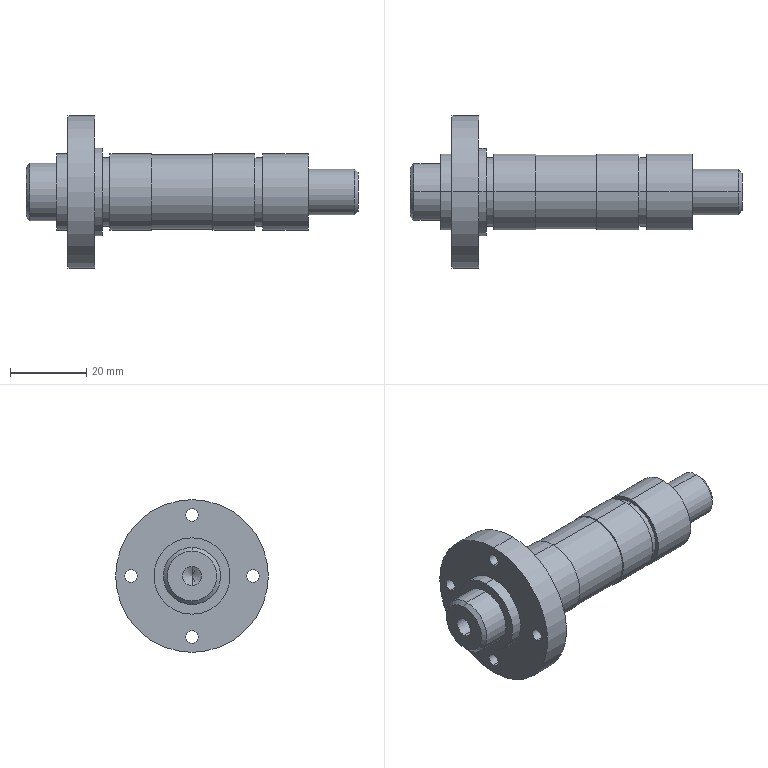Part | SolidWorks | features HoleWzd 2, Chamfer 1, RevCut 1, Revolution 1 | 1 solid | 50 faces | box 87 x 40 x 40 mm | volume 29288 mm3 | cylinder 32 | plane 12 | cone 6 | commonest cylinder face diameters 3.3 x8 20 x8 18 x4 5 x2 12 x2 15 x2
STEP:
#1=CARTESIAN_POINT('',(0.,0.,6.5));
#2=VERTEX_POINT('',#1);
#3=CARTESIAN_POINT('',(0.,0.,-6.5));
#4=VERTEX_POINT('',#3);
#5=CARTESIAN_POINT('',(0.,0.,0.));
#6=DIRECTION('',(-1.,0.,0.));
#7=DIRECTION('',(0.,0.,-1.));
#8=AXIS2_PLACEMENT_3D('',#5,#6,#7);
#9=CIRCLE('',#8,6.5);
#10=EDGE_CURVE('',#2,#4,#9,.T.);
#11=ORIENTED_EDGE('',*,*,#10,.F.);
#12=CARTESIAN_POINT('',(1.,0.,7.5));
#13=VERTEX_POINT('',#12);
#14=CARTESIAN_POINT('',(0.,0.,6.5));
#15=DIRECTION('',(0.7071,0.,0.7071));
#16=VECTOR('',#15,1000.);
#17=LINE('',#14,#16);
#18=EDGE_CURVE('',#2,#13,#17,.T.);
#19=ORIENTED_EDGE('',*,*,#18,.T.);
#20=CARTESIAN_POINT('',(1.,0.,-7.5));
#21=VERTEX_POINT('',#20);
#22=CARTESIAN_POINT('',(1.,0.,0.));
#23=DIRECTION('',(1.,0.,0.));
#24=DIRECTION('',(0.,0.,-1.));
#25=AXIS2_PLACEMENT_3D('',#22,#23,#24);
#26=CIRCLE('',#25,7.5);
#27=EDGE_CURVE('',#21,#13,#26,.T.);
#28=ORIENTED_EDGE('',*,*,#27,.F.);
#29=CARTESIAN_POINT('',(0.,0.,-6.5));
#30=DIRECTION('',(0.7071,0.,-0.7071));
#31=VECTOR('',#30,1000.);
#32=LINE('',#29,#31);
#33=EDGE_CURVE('',#4,#21,#32,.T.);
#34=ORIENTED_EDGE('',*,*,#33,.F.);
#35=EDGE_LOOP('',(#11,#19,#28,#34));
#36=FACE_OUTER_BOUND('',#35,.T.);
#37=CARTESIAN_POINT('',(0.,0.,0.));
#38=DIRECTION('',(1.,0.,0.));
#39=DIRECTION('',(0.,0.,-1.));
#40=AXIS2_PLACEMENT_3D('',#37,#38,#39);
#41=CONICAL_SURFACE('',#40,6.5,0.7854);
#42=ADVANCED_FACE('',(#36),#41,.T.);
#43=CARTESIAN_POINT('',(87.,0.,-5.));
#44=VERTEX_POINT('',#43);
#45=CARTESIAN_POINT('',(87.,0.,5.));
#46=VERTEX_POINT('',#45);
#47=CARTESIAN_POINT('',(87.,0.,0.));
#48=DIRECTION('',(1.,0.,0.));
#49=DIRECTION('',(0.,0.,1.));
#50=AXIS2_PLACEMENT_3D('',#47,#48,#49);
#51=CIRCLE('',#50,5.);
#52=EDGE_CURVE('',#44,#46,#51,.T.);
#53=ORIENTED_EDGE('',*,*,#52,.F.);
#54=CARTESIAN_POINT('',(86.,0.,-6.));
#55=VERTEX_POINT('',#54);
#56=CARTESIAN_POINT('',(86.,0.,-6.));
#57=DIRECTION('',(-0.7071,0.,-0.7071));
#58=VECTOR('',#57,1000.);
#59=LINE('',#56,#58);
#60=EDGE_CURVE('',#44,#55,#59,.T.);
#61=ORIENTED_EDGE('',*,*,#60,.T.);
#62=CARTESIAN_POINT('',(86.,0.,6.));
#63=VERTEX_POINT('',#62);
#64=CARTESIAN_POINT('',(86.,0.,0.));
#65=DIRECTION('',(-1.,0.,0.));
#66=DIRECTION('',(0.,0.,1.));
#67=AXIS2_PLACEMENT_3D('',#64,#65,#66);
#68=CIRCLE('',#67,6.);
#69=EDGE_CURVE('',#63,#55,#68,.T.);
#70=ORIENTED_EDGE('',*,*,#69,.F.);
#71=CARTESIAN_POINT('',(86.,0.,6.));
#72=DIRECTION('',(-0.7071,0.,0.7071));
#73=VECTOR('',#72,1000.);
#74=LINE('',#71,#73);
#75=EDGE_CURVE('',#46,#63,#74,.T.);
#76=ORIENTED_EDGE('',*,*,#75,.F.);
#77=EDGE_LOOP('',(#53,#61,#70,#76));
#78=FACE_OUTER_BOUND('',#77,.T.);
#79=CARTESIAN_POINT('',(86.,0.,0.));
#80=DIRECTION('',(-1.,0.,0.));
#81=DIRECTION('',(0.,0.,1.));
#82=AXIS2_PLACEMENT_3D('',#79,#80,#81);
#83=CONICAL_SURFACE('',#82,6.,0.7854);
#84=ADVANCED_FACE('',(#78),#83,.T.);
#85=CARTESIAN_POINT('',(20.,0.,11.5));
#86=VERTEX_POINT('',#85);
#87=CARTESIAN_POINT('',(20.,0.,-11.5));
#88=VERTEX_POINT('',#87);
#89=CARTESIAN_POINT('',(20.,0.,0.));
#90=DIRECTION('',(-1.,0.,0.));
#91=DIRECTION('',(0.,0.,1.));
#92=AXIS2_PLACEMENT_3D('',#89,#90,#91);
#93=CIRCLE('',#92,11.5);
#94=EDGE_CURVE('',#86,#88,#93,.T.);
#95=ORIENTED_EDGE('',*,*,#94,.T.);
#96=CARTESIAN_POINT('',(18.,0.,-11.5));
#97=VERTEX_POINT('',#96);
#98=CARTESIAN_POINT('',(0.,0.,-11.5));
#99=DIRECTION('',(-1.,0.,0.));
#100=VECTOR('',#99,1000.);
#101=LINE('',#98,#100);
#102=EDGE_CURVE('',#88,#97,#101,.T.);
#103=ORIENTED_EDGE('',*,*,#102,.T.);
#104=CARTESIAN_POINT('',(18.,0.,11.5));
#105=VERTEX_POINT('',#104);
#106=CARTESIAN_POINT('',(18.,0.,0.));
#107=DIRECTION('',(-1.,0.,0.));
#108=DIRECTION('',(0.,0.,1.));
#109=AXIS2_PLACEMENT_3D('',#106,#107,#108);
#110=CIRCLE('',#109,11.5);
#111=EDGE_CURVE('',#105,#97,#110,.T.);
#112=ORIENTED_EDGE('',*,*,#111,.F.);
#113=CARTESIAN_POINT('',(0.,0.,11.5));
#114=DIRECTION('',(-1.,0.,0.));
#115=VECTOR('',#114,1000.);
#116=LINE('',#113,#115);
#117=EDGE_CURVE('',#86,#105,#116,.T.);
#118=ORIENTED_EDGE('',*,*,#117,.F.);
#119=EDGE_LOOP('',(#95,#103,#112,#118));
#120=FACE_OUTER_BOUND('',#119,.T.);
#121=CARTESIAN_POINT('',(0.,0.,0.));
#122=DIRECTION('',(-1.,0.,0.));
#123=DIRECTION('',(0.,0.,1.));
#124=AXIS2_PLACEMENT_3D('',#121,#122,#123);
#125=CYLINDRICAL_SURFACE('',#124,11.5);
#126=ADVANCED_FACE('',(#120),#125,.T.);
#127=CARTESIAN_POINT('',(18.,16.,-1.65));
#128=VERTEX_POINT('',#127);
#129=CARTESIAN_POINT('',(18.,16.,1.65));
#130=VERTEX_POINT('',#129);
#131=CARTESIAN_POINT('',(18.,16.,0.));
#132=DIRECTION('',(-1.,0.,0.));
#133=DIRECTION('',(0.,0.,1.));
#134=AXIS2_PLACEMENT_3D('',#131,#132,#133);
#135=CIRCLE('',#134,1.65);
#136=EDGE_CURVE('',#128,#130,#135,.T.);
#137=ORIENTED_EDGE('',*,*,#136,.F.);
#138=CARTESIAN_POINT('',(11.,16.,-1.65));
#139=VERTEX_POINT('',#138);
#140=CARTESIAN_POINT('',(11.,16.,-1.65));
#141=DIRECTION('',(-1.,0.,0.));
#142=VECTOR('',#141,1000.);
#143=LINE('',#140,#142);
#144=EDGE_CURVE('',#128,#139,#143,.T.);
#145=ORIENTED_EDGE('',*,*,#144,.T.);
#146=CARTESIAN_POINT('',(11.,16.,1.65));
#147=VERTEX_POINT('',#146);
#148=CARTESIAN_POINT('',(11.,16.,0.));
#149=DIRECTION('',(-1.,0.,0.));
#150=DIRECTION('',(0.,0.,1.));
#151=AXIS2_PLACEMENT_3D('',#148,#149,#150);
#152=CIRCLE('',#151,1.65);
#153=EDGE_CURVE('',#139,#147,#152,.T.);
#154=ORIENTED_EDGE('',*,*,#153,.T.);
#155=CARTESIAN_POINT('',(11.,16.,1.65));
#156=DIRECTION('',(-1.,0.,0.));
#157=VECTOR('',#156,1000.);
#158=LINE('',#155,#157);
#159=EDGE_CURVE('',#130,#147,#158,.T.);
#160=ORIENTED_EDGE('',*,*,#159,.F.);
#161=EDGE_LOOP('',(#137,#145,#154,#160));
#162=FACE_OUTER_BOUND('',#161,.T.);
#163=CARTESIAN_POINT('',(11.,16.,0.));
#164=DIRECTION('',(-1.,0.,0.));
#165=DIRECTION('',(0.,0.,1.));
#166=AXIS2_PLACEMENT_3D('',#163,#164,#165);
#167=CYLINDRICAL_SURFACE('',#166,1.65);
#168=ADVANCED_FACE('',(#162),#167,.F.);
#169=CARTESIAN_POINT('',(18.,0.,-17.65));
#170=VERTEX_POINT('',#169);
#171=CARTESIAN_POINT('',(18.,0.,-14.35));
#172=VERTEX_POINT('',#171);
#173=CARTESIAN_POINT('',(18.,0.,-16.));
#174=DIRECTION('',(-1.,0.,0.));
#175=DIRECTION('',(0.,0.,1.));
#176=AXIS2_PLACEMENT_3D('',#173,#174,#175);
#177=CIRCLE('',#176,1.65);
#178=EDGE_CURVE('',#170,#172,#177,.T.);
#179=ORIENTED_EDGE('',*,*,#178,.F.);
#180=CARTESIAN_POINT('',(11.,0.,-17.65));
#181=VERTEX_POINT('',#180);
#182=CARTESIAN_POINT('',(11.,0.,-17.65));
#183=DIRECTION('',(-1.,0.,0.));
#184=VECTOR('',#183,1000.);
#185=LINE('',#182,#184);
#186=EDGE_CURVE('',#170,#181,#185,.T.);
#187=ORIENTED_EDGE('',*,*,#186,.T.);
#188=CARTESIAN_POINT('',(11.,0.,-14.35));
#189=VERTEX_POINT('',#188);
#190=CARTESIAN_POINT('',(11.,0.,-16.));
#191=DIRECTION('',(-1.,0.,0.));
#192=DIRECTION('',(0.,0.,1.));
#193=AXIS2_PLACEMENT_3D('',#190,#191,#192);
#194=CIRCLE('',#193,1.65);
#195=EDGE_CURVE('',#181,#189,#194,.T.);
#196=ORIENTED_EDGE('',*,*,#195,.T.);
#197=CARTESIAN_POINT('',(11.,0.,-14.35));
#198=DIRECTION('',(-1.,0.,0.));
#199=VECTOR('',#198,1000.);
#200=LINE('',#197,#199);
#201=EDGE_CURVE('',#172,#189,#200,.T.);
#202=ORIENTED_EDGE('',*,*,#201,.F.);
#203=EDGE_LOOP('',(#179,#187,#196,#202));
#204=FACE_OUTER_BOUND('',#203,.T.);
#205=CARTESIAN_POINT('',(11.,0.,-16.));
#206=DIRECTION('',(-1.,0.,0.));
#207=DIRECTION('',(0.,0.,1.));
#208=AXIS2_PLACEMENT_3D('',#205,#206,#207);
#209=CYLINDRICAL_SURFACE('',#208,1.65);
#210=ADVANCED_FACE('',(#204),#209,.F.);
#211=CARTESIAN_POINT('',(18.,-16.,-1.65));
#212=VERTEX_POINT('',#211);
#213=CARTESIAN_POINT('',(18.,-16.,1.65));
#214=VERTEX_POINT('',#213);
#215=CARTESIAN_POINT('',(18.,-16.,0.));
#216=DIRECTION('',(-1.,0.,0.));
#217=DIRECTION('',(0.,0.,1.));
#218=AXIS2_PLACEMENT_3D('',#215,#216,#217);
#219=CIRCLE('',#218,1.65);
#220=EDGE_CURVE('',#212,#214,#219,.T.);
#221=ORIENTED_EDGE('',*,*,#220,.F.);
#222=CARTESIAN_POINT('',(11.,-16.,-1.65));
#223=VERTEX_POINT('',#222);
#224=CARTESIAN_POINT('',(11.,-16.,-1.65));
#225=DIRECTION('',(-1.,0.,0.));
#226=VECTOR('',#225,1000.);
#227=LINE('',#224,#226);
#228=EDGE_CURVE('',#212,#223,#227,.T.);
#229=ORIENTED_EDGE('',*,*,#228,.T.);
#230=CARTESIAN_POINT('',(11.,-16.,1.65));
#231=VERTEX_POINT('',#230);
#232=CARTESIAN_POINT('',(11.,-16.,0.));
#233=DIRECTION('',(-1.,0.,0.));
#234=DIRECTION('',(0.,0.,1.));
#235=AXIS2_PLACEMENT_3D('',#232,#233,#234);
#236=CIRCLE('',#235,1.65);
#237=EDGE_CURVE('',#223,#231,#236,.T.);
#238=ORIENTED_EDGE('',*,*,#237,.T.);
#239=CARTESIAN_POINT('',(11.,-16.,1.65));
#240=DIRECTION('',(-1.,0.,0.));
#241=VECTOR('',#240,1000.);
#242=LINE('',#239,#241);
#243=EDGE_CURVE('',#214,#231,#242,.T.);
#244=ORIENTED_EDGE('',*,*,#243,.F.);
#245=EDGE_LOOP('',(#221,#229,#238,#244));
#246=FACE_OUTER_BOUND('',#245,.T.);
#247=CARTESIAN_POINT('',(11.,-16.,0.));
#248=DIRECTION('',(-1.,0.,0.));
#249=DIRECTION('',(0.,0.,1.));
#250=AXIS2_PLACEMENT_3D('',#247,#248,#249);
#251=CYLINDRICAL_SURFACE('',#250,1.65);
#252=ADVANCED_FACE('',(#246),#251,.F.);
#253=CARTESIAN_POINT('',(18.,0.,14.35));
#254=VERTEX_POINT('',#253);
#255=CARTESIAN_POINT('',(18.,0.,17.65));
#256=VERTEX_POINT('',#255);
#257=CARTESIAN_POINT('',(18.,0.,16.));
#258=DIRECTION('',(-1.,0.,0.));
#259=DIRECTION('',(0.,0.,1.));
#260=AXIS2_PLACEMENT_3D('',#257,#258,#259);
#261=CIRCLE('',#260,1.65);
#262=EDGE_CURVE('',#254,#256,#261,.T.);
#263=ORIENTED_EDGE('',*,*,#262,.F.);
#264=CARTESIAN_POINT('',(11.,0.,14.35));
#265=VERTEX_POINT('',#264);
#266=CARTESIAN_POINT('',(11.,0.,14.35));
#267=DIRECTION('',(-1.,0.,0.));
#268=VECTOR('',#267,1000.);
#269=LINE('',#266,#268);
#270=EDGE_CURVE('',#254,#265,#269,.T.);
#271=ORIENTED_EDGE('',*,*,#270,.T.);
#272=CARTESIAN_POINT('',(11.,0.,17.65));
#273=VERTEX_POINT('',#272);
#274=CARTESIAN_POINT('',(11.,0.,16.));
#275=DIRECTION('',(-1.,0.,0.));
#276=DIRECTION('',(0.,0.,1.));
#277=AXIS2_PLACEMENT_3D('',#274,#275,#276);
#278=CIRCLE('',#277,1.65);
#279=EDGE_CURVE('',#265,#273,#278,.T.);
#280=ORIENTED_EDGE('',*,*,#279,.T.);
#281=CARTESIAN_POINT('',(11.,0.,17.65));
#282=DIRECTION('',(-1.,0.,0.));
#283=VECTOR('',#282,1000.);
#284=LINE('',#281,#283);
#285=EDGE_CURVE('',#256,#273,#284,.T.);
#286=ORIENTED_EDGE('',*,*,#285,.F.);
#287=EDGE_LOOP('',(#263,#271,#280,#286));
#288=FACE_OUTER_BOUND('',#287,.T.);
#289=CARTESIAN_POINT('',(11.,0.,16.));
#290=DIRECTION('',(-1.,0.,0.));
#291=DIRECTION('',(0.,0.,1.));
#292=AXIS2_PLACEMENT_3D('',#289,#290,#291);
#293=CYLINDRICAL_SURFACE('',#292,1.65);
#294=ADVANCED_FACE('',(#288),#293,.F.);
#295=CARTESIAN_POINT('',(18.,0.,20.));
#296=VERTEX_POINT('',#295);
#297=CARTESIAN_POINT('',(18.,0.,-20.));
#298=VERTEX_POINT('',#297);
#299=CARTESIAN_POINT('',(18.,0.,0.));
#300=DIRECTION('',(-1.,0.,0.));
#301=DIRECTION('',(0.,0.,1.));
#302=AXIS2_PLACEMENT_3D('',#299,#300,#301);
#303=CIRCLE('',#302,20.);
#304=EDGE_CURVE('',#296,#298,#303,.T.);
#305=ORIENTED_EDGE('',*,*,#304,.T.);
#306=CARTESIAN_POINT('',(11.,0.,-20.));
#307=VERTEX_POINT('',#306);
#308=CARTESIAN_POINT('',(0.,0.,-20.));
#309=DIRECTION('',(-1.,0.,0.));
#310=VECTOR('',#309,1000.);
#311=LINE('',#308,#310);
#312=EDGE_CURVE('',#298,#307,#311,.T.);
#313=ORIENTED_EDGE('',*,*,#312,.T.);
#314=CARTESIAN_POINT('',(11.,0.,20.));
#315=VERTEX_POINT('',#314);
#316=CARTESIAN_POINT('',(11.,0.,0.));
#317=DIRECTION('',(-1.,0.,0.));
#318=DIRECTION('',(0.,0.,1.));
#319=AXIS2_PLACEMENT_3D('',#316,#317,#318);
#320=CIRCLE('',#319,20.);
#321=EDGE_CURVE('',#315,#307,#320,.T.);
#322=ORIENTED_EDGE('',*,*,#321,.F.);
#323=CARTESIAN_POINT('',(0.,0.,20.));
#324=DIRECTION('',(-1.,0.,0.));
#325=VECTOR('',#324,1000.);
#326=LINE('',#323,#325);
#327=EDGE_CURVE('',#296,#315,#326,.T.);
#328=ORIENTED_EDGE('',*,*,#327,.F.);
#329=EDGE_LOOP('',(#305,#313,#322,#328));
#330=FACE_OUTER_BOUND('',#329,.T.);
#331=CARTESIAN_POINT('',(0.,0.,0.));
#332=DIRECTION('',(-1.,0.,0.));
#333=DIRECTION('',(0.,0.,1.));
#334=AXIS2_PLACEMENT_3D('',#331,#332,#333);
#335=CYLINDRICAL_SURFACE('',#334,20.);
#336=ADVANCED_FACE('',(#330),#335,.T.);
#337=CARTESIAN_POINT('',(11.,0.,10.));
#338=VERTEX_POINT('',#337);
#339=CARTESIAN_POINT('',(11.,0.,-10.));
#340=VERTEX_POINT('',#339);
#341=CARTESIAN_POINT('',(11.,0.,0.));
#342=DIRECTION('',(-1.,0.,0.));
#343=DIRECTION('',(0.,0.,1.));
#344=AXIS2_PLACEMENT_3D('',#341,#342,#343);
#345=CIRCLE('',#344,10.);
#346=EDGE_CURVE('',#338,#340,#345,.T.);
#347=ORIENTED_EDGE('',*,*,#346,.T.);
#348=CARTESIAN_POINT('',(8.,0.,-10.));
#349=VERTEX_POINT('',#348);
#350=CARTESIAN_POINT('',(0.,0.,-10.));
#351=DIRECTION('',(-1.,0.,0.));
#352=VECTOR('',#351,1000.);
#353=LINE('',#350,#352);
#354=EDGE_CURVE('',#340,#349,#353,.T.);
#355=ORIENTED_EDGE('',*,*,#354,.T.);
#356=CARTESIAN_POINT('',(8.,0.,10.));
#357=VERTEX_POINT('',#356);
#358=CARTESIAN_POINT('',(8.,0.,0.));
#359=DIRECTION('',(-1.,0.,0.));
#360=DIRECTION('',(0.,0.,1.));
#361=AXIS2_PLACEMENT_3D('',#358,#359,#360);
#362=CIRCLE('',#361,10.);
#363=EDGE_CURVE('',#357,#349,#362,.T.);
#364=ORIENTED_EDGE('',*,*,#363,.F.);
#365=CARTESIAN_POINT('',(0.,0.,10.));
#366=DIRECTION('',(-1.,0.,0.));
#367=VECTOR('',#366,1000.);
#368=LINE('',#365,#367);
#369=EDGE_CURVE('',#338,#357,#368,.T.);
#370=ORIENTED_EDGE('',*,*,#369,.F.);
#371=EDGE_LOOP('',(#347,#355,#364,#370));
#372=FACE_OUTER_BOUND('',#371,.T.);
#373=CARTESIAN_POINT('',(0.,0.,0.));
#374=DIRECTION('',(-1.,0.,0.));
#375=DIRECTION('',(0.,0.,1.));
#376=AXIS2_PLACEMENT_3D('',#373,#374,#375);
#377=CYLINDRICAL_SURFACE('',#376,10.);
#378=ADVANCED_FACE('',(#372),#377,.T.);
#379=CARTESIAN_POINT('',(8.,0.,7.5));
#380=VERTEX_POINT('',#379);
#381=CARTESIAN_POINT('',(8.,0.,-7.5));
#382=VERTEX_POINT('',#381);
#383=CARTESIAN_POINT('',(8.,0.,0.));
#384=DIRECTION('',(-1.,0.,0.));
#385=DIRECTION('',(0.,0.,1.));
#386=AXIS2_PLACEMENT_3D('',#383,#384,#385);
#387=CIRCLE('',#386,7.5);
#388=EDGE_CURVE('',#380,#382,#387,.T.);
#389=ORIENTED_EDGE('',*,*,#388,.T.);
#390=CARTESIAN_POINT('',(0.,0.,-7.5));
#391=DIRECTION('',(-1.,0.,0.));
#392=VECTOR('',#391,1000.);
#393=LINE('',#390,#392);
#394=EDGE_CURVE('',#382,#21,#393,.T.);
#395=ORIENTED_EDGE('',*,*,#394,.T.);
#396=ORIENTED_EDGE('',*,*,#27,.T.);
#397=CARTESIAN_POINT('',(0.,0.,7.5));
#398=DIRECTION('',(-1.,0.,0.));
#399=VECTOR('',#398,1000.);
#400=LINE('',#397,#399);
#401=EDGE_CURVE('',#380,#13,#400,.T.);
#402=ORIENTED_EDGE('',*,*,#401,.F.);
#403=EDGE_LOOP('',(#389,#395,#396,#402));
#404=FACE_OUTER_BOUND('',#403,.T.);
#405=CARTESIAN_POINT('',(0.,0.,0.));
#406=DIRECTION('',(-1.,0.,0.));
#407=DIRECTION('',(0.,0.,1.));
#408=AXIS2_PLACEMENT_3D('',#405,#406,#407);
#409=CYLINDRICAL_SURFACE('',#408,7.5);
#410=ADVANCED_FACE('',(#404),#409,.T.);
#411=CARTESIAN_POINT('',(18.,0.,-2.5));
#412=VERTEX_POINT('',#411);
#413=CARTESIAN_POINT('',(18.,0.,2.5));
#414=VERTEX_POINT('',#413);
#415=CARTESIAN_POINT('',(18.,0.,0.));
#416=DIRECTION('',(-1.,0.,0.));
#417=DIRECTION('',(0.,0.,1.));
#418=AXIS2_PLACEMENT_3D('',#415,#416,#417);
#419=CIRCLE('',#418,2.5);
#420=EDGE_CURVE('',#412,#414,#419,.T.);
#421=ORIENTED_EDGE('',*,*,#420,.F.);
#422=CARTESIAN_POINT('',(0.,0.,-2.5));
#423=VERTEX_POINT('',#422);
#424=CARTESIAN_POINT('',(0.,0.,-2.5));
#425=DIRECTION('',(-1.,0.,0.));
#426=VECTOR('',#425,1000.);
#427=LINE('',#424,#426);
#428=EDGE_CURVE('',#412,#423,#427,.T.);
#429=ORIENTED_EDGE('',*,*,#428,.T.);
#430=CARTESIAN_POINT('',(0.,0.,2.5));
#431=VERTEX_POINT('',#430);
#432=CARTESIAN_POINT('',(0.,0.,0.));
#433=DIRECTION('',(-1.,0.,0.));
#434=DIRECTION('',(0.,0.,1.));
#435=AXIS2_PLACEMENT_3D('',#432,#433,#434);
#436=CIRCLE('',#435,2.5);
#437=EDGE_CURVE('',#423,#431,#436,.T.);
#438=ORIENTED_EDGE('',*,*,#437,.T.);
#439=CARTESIAN_POINT('',(0.,0.,2.5));
#440=DIRECTION('',(-1.,0.,0.));
#441=VECTOR('',#440,1000.);
#442=LINE('',#439,#441);
#443=EDGE_CURVE('',#414,#431,#442,.T.);
#444=ORIENTED_EDGE('',*,*,#443,.F.);
#445=EDGE_LOOP('',(#421,#429,#438,#444));
#446=FACE_OUTER_BOUND('',#445,.T.);
#447=CARTESIAN_POINT('',(0.,0.,0.));
#448=DIRECTION('',(-1.,0.,0.));
#449=DIRECTION('',(0.,0.,1.));
#450=AXIS2_PLACEMENT_3D('',#447,#448,#449);
#451=CYLINDRICAL_SURFACE('',#450,2.5);
#452=ADVANCED_FACE('',(#446),#451,.F.);
#453=CARTESIAN_POINT('',(19.502,0.,0.));
#454=VERTEX_POINT('',#453);
#455=CARTESIAN_POINT('',(18.,0.,2.5));
#456=DIRECTION('',(-0.515,0.,0.8572));
#457=VECTOR('',#456,1000.);
#458=LINE('',#455,#457);
#459=EDGE_CURVE('',#454,#414,#458,.T.);
#460=ORIENTED_EDGE('',*,*,#459,.F.);
#461=CARTESIAN_POINT('',(18.,0.,-2.5));
#462=DIRECTION('',(-0.515,0.,-0.8572));
#463=VECTOR('',#462,1000.);
#464=LINE('',#461,#463);
#465=EDGE_CURVE('',#454,#412,#464,.T.);
#466=ORIENTED_EDGE('',*,*,#465,.T.);
#467=ORIENTED_EDGE('',*,*,#420,.T.);
#468=EDGE_LOOP('',(#460,#466,#467));
#469=FACE_OUTER_BOUND('',#468,.T.);
#470=CARTESIAN_POINT('',(18.,0.,0.));
#471=DIRECTION('',(-1.,0.,0.));
#472=DIRECTION('',(0.,0.,1.));
#473=AXIS2_PLACEMENT_3D('',#470,#471,#472);
#474=CONICAL_SURFACE('',#473,2.5,1.03);
#475=ADVANCED_FACE('',(#469),#474,.F.);
#476=CARTESIAN_POINT('',(22.,0.,9.));
#477=VERTEX_POINT('',#476);
#478=CARTESIAN_POINT('',(22.,0.,-9.));
#479=VERTEX_POINT('',#478);
#480=CARTESIAN_POINT('',(22.,0.,0.));
#481=DIRECTION('',(-1.,0.,0.));
#482=DIRECTION('',(0.,0.,1.));
#483=AXIS2_PLACEMENT_3D('',#480,#481,#482);
#484=CIRCLE('',#483,9.);
#485=EDGE_CURVE('',#477,#479,#484,.T.);
#486=ORIENTED_EDGE('',*,*,#485,.T.);
#487=CARTESIAN_POINT('',(20.,0.,-9.));
#488=VERTEX_POINT('',#487);
#489=CARTESIAN_POINT('',(0.,0.,-9.));
#490=DIRECTION('',(-1.,0.,0.));
#491=VECTOR('',#490,1000.);
#492=LINE('',#489,#491);
#493=EDGE_CURVE('',#479,#488,#492,.T.);
#494=ORIENTED_EDGE('',*,*,#493,.T.);
#495=CARTESIAN_POINT('',(20.,0.,9.));
#496=VERTEX_POINT('',#495);
#497=CARTESIAN_POINT('',(20.,0.,0.));
#498=DIRECTION('',(-1.,0.,0.));
#499=DIRECTION('',(0.,0.,1.));
#500=AXIS2_PLACEMENT_3D('',#497,#498,#499);
#501=CIRCLE('',#500,9.);
#502=EDGE_CURVE('',#496,#488,#501,.T.);
#503=ORIENTED_EDGE('',*,*,#502,.F.);
#504=CARTESIAN_POINT('',(0.,0.,9.));
#505=DIRECTION('',(-1.,0.,0.));
#506=VECTOR('',#505,1000.);
#507=LINE('',#504,#506);
#508=EDGE_CURVE('',#477,#496,#507,.T.);
#509=ORIENTED_EDGE('',*,*,#508,.F.);
#510=EDGE_LOOP('',(#486,#494,#503,#509));
#511=FACE_OUTER_BOUND('',#510,.T.);
#512=CARTESIAN_POINT('',(0.,0.,0.));
#513=DIRECTION('',(-1.,0.,0.));
#514=DIRECTION('',(0.,0.,1.));
#515=AXIS2_PLACEMENT_3D('',#512,#513,#514);
#516=CYLINDRICAL_SURFACE('',#515,9.);
#517=ADVANCED_FACE('',(#511),#516,.T.);
#518=ORIENTED_EDGE('',*,*,#69,.T.);
#519=CARTESIAN_POINT('',(74.,0.,-6.));
#520=VERTEX_POINT('',#519);
#521=CARTESIAN_POINT('',(0.,0.,-6.));
#522=DIRECTION('',(-1.,0.,0.));
#523=VECTOR('',#522,1000.);
#524=LINE('',#521,#523);
#525=EDGE_CURVE('',#55,#520,#524,.T.);
#526=ORIENTED_EDGE('',*,*,#525,.T.);
#527=CARTESIAN_POINT('',(74.,0.,6.));
#528=VERTEX_POINT('',#527);
#529=CARTESIAN_POINT('',(74.,0.,0.));
#530=DIRECTION('',(-1.,0.,0.));
#531=DIRECTION('',(0.,0.,1.));
#532=AXIS2_PLACEMENT_3D('',#529,#530,#531);
#533=CIRCLE('',#532,6.);
#534=EDGE_CURVE('',#528,#520,#533,.T.);
#535=ORIENTED_EDGE('',*,*,#534,.F.);
#536=CARTESIAN_POINT('',(0.,0.,6.));
#537=DIRECTION('',(-1.,0.,0.));
#538=VECTOR('',#537,1000.);
#539=LINE('',#536,#538);
#540=EDGE_CURVE('',#63,#528,#539,.T.);
#541=ORIENTED_EDGE('',*,*,#540,.F.);
#542=EDGE_LOOP('',(#518,#526,#535,#541));
#543=FACE_OUTER_BOUND('',#542,.T.);
#544=CARTESIAN_POINT('',(0.,0.,0.));
#545=DIRECTION('',(-1.,0.,0.));
#546=DIRECTION('',(0.,0.,1.));
#547=AXIS2_PLACEMENT_3D('',#544,#545,#546);
#548=CYLINDRICAL_SURFACE('',#547,6.);
#549=ADVANCED_FACE('',(#543),#548,.T.);
#550=CARTESIAN_POINT('',(74.,0.,10.));
#551=VERTEX_POINT('',#550);
#552=CARTESIAN_POINT('',(74.,0.,-10.));
#553=VERTEX_POINT('',#552);
#554=CARTESIAN_POINT('',(74.,0.,0.));
#555=DIRECTION('',(-1.,0.,0.));
#556=DIRECTION('',(0.,0.,1.));
#557=AXIS2_PLACEMENT_3D('',#554,#555,#556);
#558=CIRCLE('',#557,10.);
#559=EDGE_CURVE('',#551,#553,#558,.T.);
#560=ORIENTED_EDGE('',*,*,#559,.T.);
#561=CARTESIAN_POINT('',(62.,0.,-10.));
#562=VERTEX_POINT('',#561);
#563=CARTESIAN_POINT('',(0.,0.,-10.));
#564=DIRECTION('',(-1.,0.,0.));
#565=VECTOR('',#564,1000.);
#566=LINE('',#563,#565);
#567=EDGE_CURVE('',#553,#562,#566,.T.);
#568=ORIENTED_EDGE('',*,*,#567,.T.);
#569=CARTESIAN_POINT('',(62.,0.,10.));
#570=VERTEX_POINT('',#569);
#571=CARTESIAN_POINT('',(62.,0.,0.));
#572=DIRECTION('',(-1.,0.,0.));
#573=DIRECTION('',(0.,0.,1.));
#574=AXIS2_PLACEMENT_3D('',#571,#572,#573);
#575=CIRCLE('',#574,10.);
#576=EDGE_CURVE('',#570,#562,#575,.T.);
#577=ORIENTED_EDGE('',*,*,#576,.F.);
#578=CARTESIAN_POINT('',(0.,0.,10.));
#579=DIRECTION('',(-1.,0.,0.));
#580=VECTOR('',#579,1000.);
#581=LINE('',#578,#580);
#582=EDGE_CURVE('',#551,#570,#581,.T.);
#583=ORIENTED_EDGE('',*,*,#582,.F.);
#584=EDGE_LOOP('',(#560,#568,#577,#583));
#585=FACE_OUTER_BOUND('',#584,.T.);
#586=CARTESIAN_POINT('',(0.,0.,0.));
#587=DIRECTION('',(-1.,0.,0.));
#588=DIRECTION('',(0.,0.,1.));
#589=AXIS2_PLACEMENT_3D('',#586,#587,#588);
#590=CYLINDRICAL_SURFACE('',#589,10.);
#591=ADVANCED_FACE('',(#585),#590,.T.);
#592=CARTESIAN_POINT('',(62.,0.,9.));
#593=VERTEX_POINT('',#592);
#594=CARTESIAN_POINT('',(62.,0.,-9.));
#595=VERTEX_POINT('',#594);
#596=CARTESIAN_POINT('',(62.,0.,0.));
#597=DIRECTION('',(-1.,0.,0.));
#598=DIRECTION('',(0.,0.,1.));
#599=AXIS2_PLACEMENT_3D('',#596,#597,#598);
#600=CIRCLE('',#599,9.);
#601=EDGE_CURVE('',#593,#595,#600,.T.);
#602=ORIENTED_EDGE('',*,*,#601,.T.);
#603=CARTESIAN_POINT('',(60.,0.,-9.));
#604=VERTEX_POINT('',#603);
#605=CARTESIAN_POINT('',(0.,0.,-9.));
#606=DIRECTION('',(-1.,0.,0.));
#607=VECTOR('',#606,1000.);
#608=LINE('',#605,#607);
#609=EDGE_CURVE('',#595,#604,#608,.T.);
#610=ORIENTED_EDGE('',*,*,#609,.T.);
#611=CARTESIAN_POINT('',(60.,0.,9.));
#612=VERTEX_POINT('',#611);
#613=CARTESIAN_POINT('',(60.,0.,0.));
#614=DIRECTION('',(-1.,0.,0.));
#615=DIRECTION('',(0.,0.,1.));
#616=AXIS2_PLACEMENT_3D('',#613,#614,#615);
#617=CIRCLE('',#616,9.);
#618=EDGE_CURVE('',#612,#604,#617,.T.);
#619=ORIENTED_EDGE('',*,*,#618,.F.);
#620=CARTESIAN_POINT('',(0.,0.,9.));
#621=DIRECTION('',(-1.,0.,0.));
#622=VECTOR('',#621,1000.);
#623=LINE('',#620,#622);
#624=EDGE_CURVE('',#593,#612,#623,.T.);
#625=ORIENTED_EDGE('',*,*,#624,.F.);
#626=EDGE_LOOP('',(#602,#610,#619,#625));
#627=FACE_OUTER_BOUND('',#626,.T.);
#628=CARTESIAN_POINT('',(0.,0.,0.));
#629=DIRECTION('',(-1.,0.,0.));
#630=DIRECTION('',(0.,0.,1.));
#631=AXIS2_PLACEMENT_3D('',#628,#629,#630);
#632=CYLINDRICAL_SURFACE('',#631,9.);
#633=ADVANCED_FACE('',(#627),#632,.T.);
#634=CARTESIAN_POINT('',(60.,0.,10.));
#635=VERTEX_POINT('',#634);
#636=CARTESIAN_POINT('',(60.,0.,-10.));
#637=VERTEX_POINT('',#636);
#638=CARTESIAN_POINT('',(60.,0.,0.));
#639=DIRECTION('',(-1.,0.,0.));
#640=DIRECTION('',(0.,0.,1.));
#641=AXIS2_PLACEMENT_3D('',#638,#639,#640);
#642=CIRCLE('',#641,10.);
#643=EDGE_CURVE('',#635,#637,#642,.T.);
#644=ORIENTED_EDGE('',*,*,#643,.T.);
#645=CARTESIAN_POINT('',(49.,0.,-10.));
#646=VERTEX_POINT('',#645);
#647=CARTESIAN_POINT('',(0.,0.,-10.));
#648=DIRECTION('',(-1.,0.,0.));
#649=VECTOR('',#648,1000.);
#650=LINE('',#647,#649);
#651=EDGE_CURVE('',#637,#646,#650,.T.);
#652=ORIENTED_EDGE('',*,*,#651,.T.);
#653=CARTESIAN_POINT('',(49.,0.,10.));
#654=VERTEX_POINT('',#653);
#655=CARTESIAN_POINT('',(49.,0.,0.));
#656=DIRECTION('',(-1.,0.,0.));
#657=DIRECTION('',(0.,0.,1.));
#658=AXIS2_PLACEMENT_3D('',#655,#656,#657);
#659=CIRCLE('',#658,10.);
#660=EDGE_CURVE('',#654,#646,#659,.T.);
#661=ORIENTED_EDGE('',*,*,#660,.F.);
#662=CARTESIAN_POINT('',(0.,0.,10.));
#663=DIRECTION('',(-1.,0.,0.));
#664=VECTOR('',#663,1000.);
#665=LINE('',#662,#664);
#666=EDGE_CURVE('',#635,#654,#665,.T.);
#667=ORIENTED_EDGE('',*,*,#666,.F.);
#668=EDGE_LOOP('',(#644,#652,#661,#667));
#669=FACE_OUTER_BOUND('',#668,.T.);
#670=CARTESIAN_POINT('',(0.,0.,0.));
#671=DIRECTION('',(-1.,0.,0.));
#672=DIRECTION('',(0.,0.,1.));
#673=AXIS2_PLACEMENT_3D('',#670,#671,#672);
#674=CYLINDRICAL_SURFACE('',#673,10.);
#675=ADVANCED_FACE('',(#669),#674,.T.);
#676=CARTESIAN_POINT('',(49.,0.,9.75));
#677=VERTEX_POINT('',#676);
#678=CARTESIAN_POINT('',(49.,0.,-9.75));
#679=VERTEX_POINT('',#678);
#680=CARTESIAN_POINT('',(49.,0.,0.));
#681=DIRECTION('',(-1.,0.,0.));
#682=DIRECTION('',(0.,0.,1.));
#683=AXIS2_PLACEMENT_3D('',#680,#681,#682);
#684=CIRCLE('',#683,9.75);
#685=EDGE_CURVE('',#677,#679,#684,.T.);
#686=ORIENTED_EDGE('',*,*,#685,.T.);
#687=CARTESIAN_POINT('',(33.,0.,-9.75));
#688=VERTEX_POINT('',#687);
#689=CARTESIAN_POINT('',(0.,0.,-9.75));
#690=DIRECTION('',(-1.,0.,0.));
#691=VECTOR('',#690,1000.);
#692=LINE('',#689,#691);
#693=EDGE_CURVE('',#679,#688,#692,.T.);
#694=ORIENTED_EDGE('',*,*,#693,.T.);
#695=CARTESIAN_POINT('',(33.,0.,9.75));
#696=VERTEX_POINT('',#695);
#697=CARTESIAN_POINT('',(33.,0.,0.));
#698=DIRECTION('',(-1.,0.,0.));
#699=DIRECTION('',(0.,0.,1.));
#700=AXIS2_PLACEMENT_3D('',#697,#698,#699);
#701=CIRCLE('',#700,9.75);
#702=EDGE_CURVE('',#696,#688,#701,.T.);
#703=ORIENTED_EDGE('',*,*,#702,.F.);
#704=CARTESIAN_POINT('',(0.,0.,9.75));
#705=DIRECTION('',(-1.,0.,0.));
#706=VECTOR('',#705,1000.);
#707=LINE('',#704,#706);
#708=EDGE_CURVE('',#677,#696,#707,.T.);
#709=ORIENTED_EDGE('',*,*,#708,.F.);
#710=EDGE_LOOP('',(#686,#694,#703,#709));
#711=FACE_OUTER_BOUND('',#710,.T.);
#712=CARTESIAN_POINT('',(0.,0.,0.));
#713=DIRECTION('',(-1.,0.,0.));
#714=DIRECTION('',(0.,0.,1.));
#715=AXIS2_PLACEMENT_3D('',#712,#713,#714);
#716=CYLINDRICAL_SURFACE('',#715,9.75);
#717=ADVANCED_FACE('',(#711),#716,.T.);
#718=CARTESIAN_POINT('',(33.,0.,10.));
#719=VERTEX_POINT('',#718);
#720=CARTESIAN_POINT('',(33.,0.,-10.));
#721=VERTEX_POINT('',#720);
#722=CARTESIAN_POINT('',(33.,0.,0.));
#723=DIRECTION('',(-1.,0.,0.));
#724=DIRECTION('',(0.,0.,1.));
#725=AXIS2_PLACEMENT_3D('',#722,#723,#724);
#726=CIRCLE('',#725,10.);
#727=EDGE_CURVE('',#719,#721,#726,.T.);
#728=ORIENTED_EDGE('',*,*,#727,.T.);
#729=CARTESIAN_POINT('',(22.,0.,-10.));
#730=VERTEX_POINT('',#729);
#731=CARTESIAN_POINT('',(0.,0.,-10.));
#732=DIRECTION('',(-1.,0.,0.));
#733=VECTOR('',#732,1000.);
#734=LINE('',#731,#733);
#735=EDGE_CURVE('',#721,#730,#734,.T.);
#736=ORIENTED_EDGE('',*,*,#735,.T.);
#737=CARTESIAN_POINT('',(22.,0.,10.));
#738=VERTEX_POINT('',#737);
#739=CARTESIAN_POINT('',(22.,0.,0.));
#740=DIRECTION('',(-1.,0.,0.));
#741=DIRECTION('',(0.,0.,1.));
#742=AXIS2_PLACEMENT_3D('',#739,#740,#741);
#743=CIRCLE('',#742,10.);
#744=EDGE_CURVE('',#738,#730,#743,.T.);
#745=ORIENTED_EDGE('',*,*,#744,.F.);
#746=CARTESIAN_POINT('',(0.,0.,10.));
#747=DIRECTION('',(-1.,0.,0.));
#748=VECTOR('',#747,1000.);
#749=LINE('',#746,#748);
#750=EDGE_CURVE('',#719,#738,#749,.T.);
#751=ORIENTED_EDGE('',*,*,#750,.F.);
#752=EDGE_LOOP('',(#728,#736,#745,#751));
#753=FACE_OUTER_BOUND('',#752,.T.);
#754=CARTESIAN_POINT('',(0.,0.,0.));
#755=DIRECTION('',(-1.,0.,0.));
#756=DIRECTION('',(0.,0.,1.));
#757=AXIS2_PLACEMENT_3D('',#754,#755,#756);
#758=CYLINDRICAL_SURFACE('',#757,10.);
#759=ADVANCED_FACE('',(#753),#758,.T.);
#760=ORIENTED_EDGE('',*,*,#735,.F.);
#761=CARTESIAN_POINT('',(33.,0.,0.));
#762=DIRECTION('',(-1.,0.,0.));
#763=DIRECTION('',(0.,0.,1.));
#764=AXIS2_PLACEMENT_3D('',#761,#762,#763);
#765=CIRCLE('',#764,10.);
#766=EDGE_CURVE('',#721,#719,#765,.T.);
#767=ORIENTED_EDGE('',*,*,#766,.T.);
#768=ORIENTED_EDGE('',*,*,#750,.T.);
#769=CARTESIAN_POINT('',(22.,0.,0.));
#770=DIRECTION('',(-1.,0.,0.));
#771=DIRECTION('',(0.,0.,1.));
#772=AXIS2_PLACEMENT_3D('',#769,#770,#771);
#773=CIRCLE('',#772,10.);
#774=EDGE_CURVE('',#730,#738,#773,.T.);
#775=ORIENTED_EDGE('',*,*,#774,.F.);
#776=EDGE_LOOP('',(#760,#767,#768,#775));
#777=FACE_OUTER_BOUND('',#776,.T.);
#778=CARTESIAN_POINT('',(0.,0.,0.));
#779=DIRECTION('',(-1.,0.,0.));
#780=DIRECTION('',(0.,0.,1.));
#781=AXIS2_PLACEMENT_3D('',#778,#779,#780);
#782=CYLINDRICAL_SURFACE('',#781,10.);
#783=ADVANCED_FACE('',(#777),#782,.T.);
#784=ORIENTED_EDGE('',*,*,#727,.F.);
#785=ORIENTED_EDGE('',*,*,#766,.F.);
#786=EDGE_LOOP('',(#784,#785));
#787=FACE_OUTER_BOUND('',#786,.T.);
#788=ORIENTED_EDGE('',*,*,#702,.T.);
#789=CARTESIAN_POINT('',(33.,0.,0.));
#790=DIRECTION('',(-1.,0.,0.));
#791=DIRECTION('',(0.,0.,1.));
#792=AXIS2_PLACEMENT_3D('',#789,#790,#791);
#793=CIRCLE('',#792,9.75);
#794=EDGE_CURVE('',#688,#696,#793,.T.);
#795=ORIENTED_EDGE('',*,*,#794,.T.);
#796=EDGE_LOOP('',(#788,#795));
#797=FACE_BOUND('',#796,.T.);
#798=CARTESIAN_POINT('',(33.,10.,0.));
#799=DIRECTION('',(-1.,0.,0.));
#800=DIRECTION('',(0.,0.,1.));
#801=AXIS2_PLACEMENT_3D('',#798,#799,#800);
#802=PLANE('',#801);
#803=ADVANCED_FACE('',(#787,#797),#802,.F.);
#804=ORIENTED_EDGE('',*,*,#693,.F.);
#805=CARTESIAN_POINT('',(49.,0.,0.));
#806=DIRECTION('',(-1.,0.,0.));
#807=DIRECTION('',(0.,0.,1.));
#808=AXIS2_PLACEMENT_3D('',#805,#806,#807);
#809=CIRCLE('',#808,9.75);
#810=EDGE_CURVE('',#679,#677,#809,.T.);
#811=ORIENTED_EDGE('',*,*,#810,.T.);
#812=ORIENTED_EDGE('',*,*,#708,.T.);
#813=ORIENTED_EDGE('',*,*,#794,.F.);
#814=EDGE_LOOP('',(#804,#811,#812,#813));
#815=FACE_OUTER_BOUND('',#814,.T.);
#816=CARTESIAN_POINT('',(0.,0.,0.));
#817=DIRECTION('',(-1.,0.,0.));
#818=DIRECTION('',(0.,0.,1.));
#819=AXIS2_PLACEMENT_3D('',#816,#817,#818);
#820=CYLINDRICAL_SURFACE('',#819,9.75);
#821=ADVANCED_FACE('',(#815),#820,.T.);
#822=ORIENTED_EDGE('',*,*,#685,.F.);
#823=ORIENTED_EDGE('',*,*,#810,.F.);
#824=EDGE_LOOP('',(#822,#823));
#825=FACE_BOUND('',#824,.T.);
#826=ORIENTED_EDGE('',*,*,#660,.T.);
#827=CARTESIAN_POINT('',(49.,0.,0.));
#828=DIRECTION('',(-1.,0.,0.));
#829=DIRECTION('',(0.,0.,1.));
#830=AXIS2_PLACEMENT_3D('',#827,#828,#829);
#831=CIRCLE('',#830,10.);
#832=EDGE_CURVE('',#646,#654,#831,.T.);
#833=ORIENTED_EDGE('',*,*,#832,.T.);
#834=EDGE_LOOP('',(#826,#833));
#835=FACE_OUTER_BOUND('',#834,.T.);
#836=CARTESIAN_POINT('',(49.,9.75,0.));
#837=DIRECTION('',(1.,0.,0.));
#838=DIRECTION('',(0.,0.,-1.));
#839=AXIS2_PLACEMENT_3D('',#836,#837,#838);
#840=PLANE('',#839);
#841=ADVANCED_FACE('',(#825,#835),#840,.F.);
#842=ORIENTED_EDGE('',*,*,#651,.F.);
#843=CARTESIAN_POINT('',(60.,0.,0.));
#844=DIRECTION('',(-1.,0.,0.));
#845=DIRECTION('',(0.,0.,1.));
#846=AXIS2_PLACEMENT_3D('',#843,#844,#845);
#847=CIRCLE('',#846,10.);
#848=EDGE_CURVE('',#637,#635,#847,.T.);
#849=ORIENTED_EDGE('',*,*,#848,.T.);
#850=ORIENTED_EDGE('',*,*,#666,.T.);
#851=ORIENTED_EDGE('',*,*,#832,.F.);
#852=EDGE_LOOP('',(#842,#849,#850,#851));
#853=FACE_OUTER_BOUND('',#852,.T.);
#854=CARTESIAN_POINT('',(0.,0.,0.));
#855=DIRECTION('',(-1.,0.,0.));
#856=DIRECTION('',(0.,0.,1.));
#857=AXIS2_PLACEMENT_3D('',#854,#855,#856);
#858=CYLINDRICAL_SURFACE('',#857,10.);
#859=ADVANCED_FACE('',(#853),#858,.T.);
#860=ORIENTED_EDGE('',*,*,#643,.F.);
#861=ORIENTED_EDGE('',*,*,#848,.F.);
#862=EDGE_LOOP('',(#860,#861));
#863=FACE_OUTER_BOUND('',#862,.T.);
#864=ORIENTED_EDGE('',*,*,#618,.T.);
#865=CARTESIAN_POINT('',(60.,0.,0.));
#866=DIRECTION('',(-1.,0.,0.));
#867=DIRECTION('',(0.,0.,1.));
#868=AXIS2_PLACEMENT_3D('',#865,#866,#867);
#869=CIRCLE('',#868,9.);
#870=EDGE_CURVE('',#604,#612,#869,.T.);
#871=ORIENTED_EDGE('',*,*,#870,.T.);
#872=EDGE_LOOP('',(#864,#871));
#873=FACE_BOUND('',#872,.T.);
#874=CARTESIAN_POINT('',(60.,10.,0.));
#875=DIRECTION('',(-1.,0.,0.));
#876=DIRECTION('',(0.,0.,1.));
#877=AXIS2_PLACEMENT_3D('',#874,#875,#876);
#878=PLANE('',#877);
#879=ADVANCED_FACE('',(#863,#873),#878,.F.);
#880=ORIENTED_EDGE('',*,*,#609,.F.);
#881=CARTESIAN_POINT('',(62.,0.,0.));
#882=DIRECTION('',(-1.,0.,0.));
#883=DIRECTION('',(0.,0.,1.));
#884=AXIS2_PLACEMENT_3D('',#881,#882,#883);
#885=CIRCLE('',#884,9.);
#886=EDGE_CURVE('',#595,#593,#885,.T.);
#887=ORIENTED_EDGE('',*,*,#886,.T.);
#888=ORIENTED_EDGE('',*,*,#624,.T.);
#889=ORIENTED_EDGE('',*,*,#870,.F.);
#890=EDGE_LOOP('',(#880,#887,#888,#889));
#891=FACE_OUTER_BOUND('',#890,.T.);
#892=CARTESIAN_POINT('',(0.,0.,0.));
#893=DIRECTION('',(-1.,0.,0.));
#894=DIRECTION('',(0.,0.,1.));
#895=AXIS2_PLACEMENT_3D('',#892,#893,#894);
#896=CYLINDRICAL_SURFACE('',#895,9.);
#897=ADVANCED_FACE('',(#891),#896,.T.);
#898=ORIENTED_EDGE('',*,*,#601,.F.);
#899=ORIENTED_EDGE('',*,*,#886,.F.);
#900=EDGE_LOOP('',(#898,#899));
#901=FACE_BOUND('',#900,.T.);
#902=ORIENTED_EDGE('',*,*,#576,.T.);
#903=CARTESIAN_POINT('',(62.,0.,0.));
#904=DIRECTION('',(-1.,0.,0.));
#905=DIRECTION('',(0.,0.,1.));
#906=AXIS2_PLACEMENT_3D('',#903,#904,#905);
#907=CIRCLE('',#906,10.);
#908=EDGE_CURVE('',#562,#570,#907,.T.);
#909=ORIENTED_EDGE('',*,*,#908,.T.);
#910=EDGE_LOOP('',(#902,#909));
#911=FACE_OUTER_BOUND('',#910,.T.);
#912=CARTESIAN_POINT('',(62.,9.,0.));
#913=DIRECTION('',(1.,0.,0.));
#914=DIRECTION('',(0.,0.,-1.));
#915=AXIS2_PLACEMENT_3D('',#912,#913,#914);
#916=PLANE('',#915);
#917=ADVANCED_FACE('',(#901,#911),#916,.F.);
#918=ORIENTED_EDGE('',*,*,#567,.F.);
#919=CARTESIAN_POINT('',(74.,0.,0.));
#920=DIRECTION('',(-1.,0.,0.));
#921=DIRECTION('',(0.,0.,1.));
#922=AXIS2_PLACEMENT_3D('',#919,#920,#921);
#923=CIRCLE('',#922,10.);
#924=EDGE_CURVE('',#553,#551,#923,.T.);
#925=ORIENTED_EDGE('',*,*,#924,.T.);
#926=ORIENTED_EDGE('',*,*,#582,.T.);
#927=ORIENTED_EDGE('',*,*,#908,.F.);
#928=EDGE_LOOP('',(#918,#925,#926,#927));
#929=FACE_OUTER_BOUND('',#928,.T.);
#930=CARTESIAN_POINT('',(0.,0.,0.));
#931=DIRECTION('',(-1.,0.,0.));
#932=DIRECTION('',(0.,0.,1.));
#933=AXIS2_PLACEMENT_3D('',#930,#931,#932);
#934=CYLINDRICAL_SURFACE('',#933,10.);
#935=ADVANCED_FACE('',(#929),#934,.T.);
#936=ORIENTED_EDGE('',*,*,#559,.F.);
#937=ORIENTED_EDGE('',*,*,#924,.F.);
#938=EDGE_LOOP('',(#936,#937));
#939=FACE_OUTER_BOUND('',#938,.T.);
#940=ORIENTED_EDGE('',*,*,#534,.T.);
#941=CARTESIAN_POINT('',(74.,0.,0.));
#942=DIRECTION('',(-1.,0.,0.));
#943=DIRECTION('',(0.,0.,1.));
#944=AXIS2_PLACEMENT_3D('',#941,#942,#943);
#945=CIRCLE('',#944,6.);
#946=EDGE_CURVE('',#520,#528,#945,.T.);
#947=ORIENTED_EDGE('',*,*,#946,.T.);
#948=EDGE_LOOP('',(#940,#947));
#949=FACE_BOUND('',#948,.T.);
#950=CARTESIAN_POINT('',(74.,10.,0.));
#951=DIRECTION('',(-1.,0.,0.));
#952=DIRECTION('',(0.,0.,1.));
#953=AXIS2_PLACEMENT_3D('',#950,#951,#952);
#954=PLANE('',#953);
#955=ADVANCED_FACE('',(#939,#949),#954,.F.);
#956=ORIENTED_EDGE('',*,*,#525,.F.);
#957=CARTESIAN_POINT('',(86.,0.,0.));
#958=DIRECTION('',(-1.,0.,0.));
#959=DIRECTION('',(0.,0.,1.));
#960=AXIS2_PLACEMENT_3D('',#957,#958,#959);
#961=CIRCLE('',#960,6.);
#962=EDGE_CURVE('',#55,#63,#961,.T.);
#963=ORIENTED_EDGE('',*,*,#962,.T.);
#964=ORIENTED_EDGE('',*,*,#540,.T.);
#965=ORIENTED_EDGE('',*,*,#946,.F.);
#966=EDGE_LOOP('',(#956,#963,#964,#965));
#967=FACE_OUTER_BOUND('',#966,.T.);
#968=CARTESIAN_POINT('',(0.,0.,0.));
#969=DIRECTION('',(-1.,0.,0.));
#970=DIRECTION('',(0.,0.,1.));
#971=AXIS2_PLACEMENT_3D('',#968,#969,#970);
#972=CYLINDRICAL_SURFACE('',#971,6.);
#973=ADVANCED_FACE('',(#967),#972,.T.);
#974=CARTESIAN_POINT('',(87.,0.,0.));
#975=DIRECTION('',(1.,0.,0.));
#976=DIRECTION('',(0.,0.,1.));
#977=AXIS2_PLACEMENT_3D('',#974,#975,#976);
#978=CIRCLE('',#977,5.);
#979=EDGE_CURVE('',#46,#44,#978,.T.);
#980=ORIENTED_EDGE('',*,*,#979,.T.);
#981=ORIENTED_EDGE('',*,*,#52,.T.);
#982=EDGE_LOOP('',(#980,#981));
#983=FACE_OUTER_BOUND('',#982,.T.);
#984=CARTESIAN_POINT('',(87.,6.,0.));
#985=DIRECTION('',(-1.,0.,0.));
#986=DIRECTION('',(0.,0.,1.));
#987=AXIS2_PLACEMENT_3D('',#984,#985,#986);
#988=PLANE('',#987);
#989=ADVANCED_FACE('',(#983),#988,.F.);
#990=ORIENTED_EDGE('',*,*,#493,.F.);
#991=CARTESIAN_POINT('',(22.,0.,0.));
#992=DIRECTION('',(-1.,0.,0.));
#993=DIRECTION('',(0.,0.,1.));
#994=AXIS2_PLACEMENT_3D('',#991,#992,#993);
#995=CIRCLE('',#994,9.);
#996=EDGE_CURVE('',#479,#477,#995,.T.);
#997=ORIENTED_EDGE('',*,*,#996,.T.);
#998=ORIENTED_EDGE('',*,*,#508,.T.);
#999=CARTESIAN_POINT('',(20.,0.,0.));
#1000=DIRECTION('',(-1.,0.,0.));
#1001=DIRECTION('',(0.,0.,1.));
#1002=AXIS2_PLACEMENT_3D('',#999,#1000,#1001);
#1003=CIRCLE('',#1002,9.);
#1004=EDGE_CURVE('',#488,#496,#1003,.T.);
#1005=ORIENTED_EDGE('',*,*,#1004,.F.);
#1006=EDGE_LOOP('',(#990,#997,#998,#1005));
#1007=FACE_OUTER_BOUND('',#1006,.T.);
#1008=CARTESIAN_POINT('',(0.,0.,0.));
#1009=DIRECTION('',(-1.,0.,0.));
#1010=DIRECTION('',(0.,0.,1.));
#1011=AXIS2_PLACEMENT_3D('',#1008,#1009,#1010);
#1012=CYLINDRICAL_SURFACE('',#1011,9.);
#1013=ADVANCED_FACE('',(#1007),#1012,.T.);
#1014=ORIENTED_EDGE('',*,*,#744,.T.);
#1015=ORIENTED_EDGE('',*,*,#774,.T.);
#1016=EDGE_LOOP('',(#1014,#1015));
#1017=FACE_OUTER_BOUND('',#1016,.T.);
#1018=ORIENTED_EDGE('',*,*,#485,.F.);
#1019=ORIENTED_EDGE('',*,*,#996,.F.);
#1020=EDGE_LOOP('',(#1018,#1019));
#1021=FACE_BOUND('',#1020,.T.);
#1022=CARTESIAN_POINT('',(22.,10.,0.));
#1023=DIRECTION('',(-1.,0.,0.));
#1024=DIRECTION('',(0.,0.,1.));
#1025=AXIS2_PLACEMENT_3D('',#1022,#1023,#1024);
#1026=PLANE('',#1025);
#1027=ADVANCED_FACE('',(#1017,#1021),#1026,.T.);
#1028=ORIENTED_EDGE('',*,*,#465,.F.);
#1029=ORIENTED_EDGE('',*,*,#459,.T.);
#1030=CARTESIAN_POINT('',(18.,0.,0.));
#1031=DIRECTION('',(-1.,0.,0.));
#1032=DIRECTION('',(0.,0.,1.));
#1033=AXIS2_PLACEMENT_3D('',#1030,#1031,#1032);
#1034=CIRCLE('',#1033,2.5);
#1035=EDGE_CURVE('',#414,#412,#1034,.T.);
#1036=ORIENTED_EDGE('',*,*,#1035,.T.);
#1037=EDGE_LOOP('',(#1028,#1029,#1036));
#1038=FACE_OUTER_BOUND('',#1037,.T.);
#1039=CARTESIAN_POINT('',(18.,0.,0.));
#1040=DIRECTION('',(-1.,0.,0.));
#1041=DIRECTION('',(0.,0.,1.));
#1042=AXIS2_PLACEMENT_3D('',#1039,#1040,#1041);
#1043=CONICAL_SURFACE('',#1042,2.5,1.03);
#1044=ADVANCED_FACE('',(#1038),#1043,.F.);
#1045=ORIENTED_EDGE('',*,*,#428,.F.);
#1046=ORIENTED_EDGE('',*,*,#1035,.F.);
#1047=ORIENTED_EDGE('',*,*,#443,.T.);
#1048=CARTESIAN_POINT('',(0.,0.,0.));
#1049=DIRECTION('',(-1.,0.,0.));
#1050=DIRECTION('',(0.,0.,1.));
#1051=AXIS2_PLACEMENT_3D('',#1048,#1049,#1050);
#1052=CIRCLE('',#1051,2.5);
#1053=EDGE_CURVE('',#431,#423,#1052,.T.);
#1054=ORIENTED_EDGE('',*,*,#1053,.T.);
#1055=EDGE_LOOP('',(#1045,#1046,#1047,#1054));
#1056=FACE_OUTER_BOUND('',#1055,.T.);
#1057=CARTESIAN_POINT('',(0.,0.,0.));
#1058=DIRECTION('',(-1.,0.,0.));
#1059=DIRECTION('',(0.,0.,1.));
#1060=AXIS2_PLACEMENT_3D('',#1057,#1058,#1059);
#1061=CYLINDRICAL_SURFACE('',#1060,2.5);
#1062=ADVANCED_FACE('',(#1056),#1061,.F.);
#1063=CARTESIAN_POINT('',(0.,0.,0.));
#1064=DIRECTION('',(-1.,0.,0.));
#1065=DIRECTION('',(0.,0.,-1.));
#1066=AXIS2_PLACEMENT_3D('',#1063,#1064,#1065);
#1067=CIRCLE('',#1066,6.5);
#1068=EDGE_CURVE('',#4,#2,#1067,.T.);
#1069=ORIENTED_EDGE('',*,*,#1068,.T.);
#1070=ORIENTED_EDGE('',*,*,#10,.T.);
#1071=EDGE_LOOP('',(#1069,#1070));
#1072=FACE_OUTER_BOUND('',#1071,.T.);
#1073=ORIENTED_EDGE('',*,*,#1053,.F.);
#1074=ORIENTED_EDGE('',*,*,#437,.F.);
#1075=EDGE_LOOP('',(#1073,#1074));
#1076=FACE_BOUND('',#1075,.T.);
#1077=CARTESIAN_POINT('',(0.,0.,0.));
#1078=DIRECTION('',(1.,0.,0.));
#1079=DIRECTION('',(0.,0.,-1.));
#1080=AXIS2_PLACEMENT_3D('',#1077,#1078,#1079);
#1081=PLANE('',#1080);
#1082=ADVANCED_FACE('',(#1072,#1076),#1081,.F.);
#1083=ORIENTED_EDGE('',*,*,#394,.F.);
#1084=CARTESIAN_POINT('',(8.,0.,0.));
#1085=DIRECTION('',(-1.,0.,0.));
#1086=DIRECTION('',(0.,0.,1.));
#1087=AXIS2_PLACEMENT_3D('',#1084,#1085,#1086);
#1088=CIRCLE('',#1087,7.5);
#1089=EDGE_CURVE('',#382,#380,#1088,.T.);
#1090=ORIENTED_EDGE('',*,*,#1089,.T.);
#1091=ORIENTED_EDGE('',*,*,#401,.T.);
#1092=CARTESIAN_POINT('',(1.,0.,0.));
#1093=DIRECTION('',(1.,0.,0.));
#1094=DIRECTION('',(0.,0.,-1.));
#1095=AXIS2_PLACEMENT_3D('',#1092,#1093,#1094);
#1096=CIRCLE('',#1095,7.5);
#1097=EDGE_CURVE('',#13,#21,#1096,.T.);
#1098=ORIENTED_EDGE('',*,*,#1097,.T.);
#1099=EDGE_LOOP('',(#1083,#1090,#1091,#1098));
#1100=FACE_OUTER_BOUND('',#1099,.T.);
#1101=CARTESIAN_POINT('',(0.,0.,0.));
#1102=DIRECTION('',(-1.,0.,0.));
#1103=DIRECTION('',(0.,0.,1.));
#1104=AXIS2_PLACEMENT_3D('',#1101,#1102,#1103);
#1105=CYLINDRICAL_SURFACE('',#1104,7.5);
#1106=ADVANCED_FACE('',(#1100),#1105,.T.);
#1107=ORIENTED_EDGE('',*,*,#388,.F.);
#1108=ORIENTED_EDGE('',*,*,#1089,.F.);
#1109=EDGE_LOOP('',(#1107,#1108));
#1110=FACE_BOUND('',#1109,.T.);
#1111=ORIENTED_EDGE('',*,*,#363,.T.);
#1112=CARTESIAN_POINT('',(8.,0.,0.));
#1113=DIRECTION('',(-1.,0.,0.));
#1114=DIRECTION('',(0.,0.,1.));
#1115=AXIS2_PLACEMENT_3D('',#1112,#1113,#1114);
#1116=CIRCLE('',#1115,10.);
#1117=EDGE_CURVE('',#349,#357,#1116,.T.);
#1118=ORIENTED_EDGE('',*,*,#1117,.T.);
#1119=EDGE_LOOP('',(#1111,#1118));
#1120=FACE_OUTER_BOUND('',#1119,.T.);
#1121=CARTESIAN_POINT('',(8.,7.5,0.));
#1122=DIRECTION('',(1.,0.,0.));
#1123=DIRECTION('',(0.,0.,-1.));
#1124=AXIS2_PLACEMENT_3D('',#1121,#1122,#1123);
#1125=PLANE('',#1124);
#1126=ADVANCED_FACE('',(#1110,#1120),#1125,.F.);
#1127=ORIENTED_EDGE('',*,*,#354,.F.);
#1128=CARTESIAN_POINT('',(11.,0.,0.));
#1129=DIRECTION('',(-1.,0.,0.));
#1130=DIRECTION('',(0.,0.,1.));
#1131=AXIS2_PLACEMENT_3D('',#1128,#1129,#1130);
#1132=CIRCLE('',#1131,10.);
#1133=EDGE_CURVE('',#340,#338,#1132,.T.);
#1134=ORIENTED_EDGE('',*,*,#1133,.T.);
#1135=ORIENTED_EDGE('',*,*,#369,.T.);
#1136=ORIENTED_EDGE('',*,*,#1117,.F.);
#1137=EDGE_LOOP('',(#1127,#1134,#1135,#1136));
#1138=FACE_OUTER_BOUND('',#1137,.T.);
#1139=CARTESIAN_POINT('',(0.,0.,0.));
#1140=DIRECTION('',(-1.,0.,0.));
#1141=DIRECTION('',(0.,0.,1.));
#1142=AXIS2_PLACEMENT_3D('',#1139,#1140,#1141);
#1143=CYLINDRICAL_SURFACE('',#1142,10.);
#1144=ADVANCED_FACE('',(#1138),#1143,.T.);
#1145=CARTESIAN_POINT('',(11.,16.,0.));
#1146=DIRECTION('',(-1.,0.,0.));
#1147=DIRECTION('',(0.,0.,1.));
#1148=AXIS2_PLACEMENT_3D('',#1145,#1146,#1147);
#1149=CIRCLE('',#1148,1.65);
#1150=EDGE_CURVE('',#147,#139,#1149,.T.);
#1151=ORIENTED_EDGE('',*,*,#1150,.F.);
#1152=ORIENTED_EDGE('',*,*,#153,.F.);
#1153=EDGE_LOOP('',(#1151,#1152));
#1154=FACE_BOUND('',#1153,.T.);
#1155=CARTESIAN_POINT('',(11.,0.,-16.));
#1156=DIRECTION('',(-1.,0.,0.));
#1157=DIRECTION('',(0.,0.,1.));
#1158=AXIS2_PLACEMENT_3D('',#1155,#1156,#1157);
#1159=CIRCLE('',#1158,1.65);
#1160=EDGE_CURVE('',#189,#181,#1159,.T.);
#1161=ORIENTED_EDGE('',*,*,#1160,.F.);
#1162=ORIENTED_EDGE('',*,*,#195,.F.);
#1163=EDGE_LOOP('',(#1161,#1162));
#1164=FACE_BOUND('',#1163,.T.);
#1165=CARTESIAN_POINT('',(11.,-16.,0.));
#1166=DIRECTION('',(-1.,0.,0.));
#1167=DIRECTION('',(0.,0.,1.));
#1168=AXIS2_PLACEMENT_3D('',#1165,#1166,#1167);
#1169=CIRCLE('',#1168,1.65);
#1170=EDGE_CURVE('',#231,#223,#1169,.T.);
#1171=ORIENTED_EDGE('',*,*,#1170,.F.);
#1172=ORIENTED_EDGE('',*,*,#237,.F.);
#1173=EDGE_LOOP('',(#1171,#1172));
#1174=FACE_BOUND('',#1173,.T.);
#1175=CARTESIAN_POINT('',(11.,0.,16.));
#1176=DIRECTION('',(-1.,0.,0.));
#1177=DIRECTION('',(0.,0.,1.));
#1178=AXIS2_PLACEMENT_3D('',#1175,#1176,#1177);
#1179=CIRCLE('',#1178,1.65);
#1180=EDGE_CURVE('',#273,#265,#1179,.T.);
#1181=ORIENTED_EDGE('',*,*,#1180,.F.);
#1182=ORIENTED_EDGE('',*,*,#279,.F.);
#1183=EDGE_LOOP('',(#1181,#1182));
#1184=FACE_BOUND('',#1183,.T.);
#1185=ORIENTED_EDGE('',*,*,#346,.F.);
#1186=ORIENTED_EDGE('',*,*,#1133,.F.);
#1187=EDGE_LOOP('',(#1185,#1186));
#1188=FACE_BOUND('',#1187,.T.);
#1189=ORIENTED_EDGE('',*,*,#321,.T.);
#1190=CARTESIAN_POINT('',(11.,0.,0.));
#1191=DIRECTION('',(-1.,0.,0.));
#1192=DIRECTION('',(0.,0.,1.));
#1193=AXIS2_PLACEMENT_3D('',#1190,#1191,#1192);
#1194=CIRCLE('',#1193,20.);
#1195=EDGE_CURVE('',#307,#315,#1194,.T.);
#1196=ORIENTED_EDGE('',*,*,#1195,.T.);
#1197=EDGE_LOOP('',(#1189,#1196));
#1198=FACE_OUTER_BOUND('',#1197,.T.);
#1199=CARTESIAN_POINT('',(11.,10.,0.));
#1200=DIRECTION('',(1.,0.,0.));
#1201=DIRECTION('',(0.,0.,-1.));
#1202=AXIS2_PLACEMENT_3D('',#1199,#1200,#1201);
#1203=PLANE('',#1202);
#1204=ADVANCED_FACE('',(#1154,#1164,#1174,#1184,#1188,#1198),#1203,.F.);
#1205=ORIENTED_EDGE('',*,*,#312,.F.);
#1206=CARTESIAN_POINT('',(18.,0.,0.));
#1207=DIRECTION('',(-1.,0.,0.));
#1208=DIRECTION('',(0.,0.,1.));
#1209=AXIS2_PLACEMENT_3D('',#1206,#1207,#1208);
#1210=CIRCLE('',#1209,20.);
#1211=EDGE_CURVE('',#298,#296,#1210,.T.);
#1212=ORIENTED_EDGE('',*,*,#1211,.T.);
#1213=ORIENTED_EDGE('',*,*,#327,.T.);
#1214=ORIENTED_EDGE('',*,*,#1195,.F.);
#1215=EDGE_LOOP('',(#1205,#1212,#1213,#1214));
#1216=FACE_OUTER_BOUND('',#1215,.T.);
#1217=CARTESIAN_POINT('',(0.,0.,0.));
#1218=DIRECTION('',(-1.,0.,0.));
#1219=DIRECTION('',(0.,0.,1.));
#1220=AXIS2_PLACEMENT_3D('',#1217,#1218,#1219);
#1221=CYLINDRICAL_SURFACE('',#1220,20.);
#1222=ADVANCED_FACE('',(#1216),#1221,.T.);
#1223=ORIENTED_EDGE('',*,*,#270,.F.);
#1224=CARTESIAN_POINT('',(18.,0.,16.));
#1225=DIRECTION('',(-1.,0.,0.));
#1226=DIRECTION('',(0.,0.,1.));
#1227=AXIS2_PLACEMENT_3D('',#1224,#1225,#1226);
#1228=CIRCLE('',#1227,1.65);
#1229=EDGE_CURVE('',#256,#254,#1228,.T.);
#1230=ORIENTED_EDGE('',*,*,#1229,.F.);
#1231=ORIENTED_EDGE('',*,*,#285,.T.);
#1232=ORIENTED_EDGE('',*,*,#1180,.T.);
#1233=EDGE_LOOP('',(#1223,#1230,#1231,#1232));
#1234=FACE_OUTER_BOUND('',#1233,.T.);
#1235=CARTESIAN_POINT('',(11.,0.,16.));
#1236=DIRECTION('',(-1.,0.,0.));
#1237=DIRECTION('',(0.,0.,1.));
#1238=AXIS2_PLACEMENT_3D('',#1235,#1236,#1237);
#1239=CYLINDRICAL_SURFACE('',#1238,1.65);
#1240=ADVANCED_FACE('',(#1234),#1239,.F.);
#1241=ORIENTED_EDGE('',*,*,#228,.F.);
#1242=CARTESIAN_POINT('',(18.,-16.,0.));
#1243=DIRECTION('',(-1.,0.,0.));
#1244=DIRECTION('',(0.,0.,1.));
#1245=AXIS2_PLACEMENT_3D('',#1242,#1243,#1244);
#1246=CIRCLE('',#1245,1.65);
#1247=EDGE_CURVE('',#214,#212,#1246,.T.);
#1248=ORIENTED_EDGE('',*,*,#1247,.F.);
#1249=ORIENTED_EDGE('',*,*,#243,.T.);
#1250=ORIENTED_EDGE('',*,*,#1170,.T.);
#1251=EDGE_LOOP('',(#1241,#1248,#1249,#1250));
#1252=FACE_OUTER_BOUND('',#1251,.T.);
#1253=CARTESIAN_POINT('',(11.,-16.,0.));
#1254=DIRECTION('',(-1.,0.,0.));
#1255=DIRECTION('',(0.,0.,1.));
#1256=AXIS2_PLACEMENT_3D('',#1253,#1254,#1255);
#1257=CYLINDRICAL_SURFACE('',#1256,1.65);
#1258=ADVANCED_FACE('',(#1252),#1257,.F.);
#1259=ORIENTED_EDGE('',*,*,#186,.F.);
#1260=CARTESIAN_POINT('',(18.,0.,-16.));
#1261=DIRECTION('',(-1.,0.,0.));
#1262=DIRECTION('',(0.,0.,1.));
#1263=AXIS2_PLACEMENT_3D('',#1260,#1261,#1262);
#1264=CIRCLE('',#1263,1.65);
#1265=EDGE_CURVE('',#172,#170,#1264,.T.);
#1266=ORIENTED_EDGE('',*,*,#1265,.F.);
#1267=ORIENTED_EDGE('',*,*,#201,.T.);
#1268=ORIENTED_EDGE('',*,*,#1160,.T.);
#1269=EDGE_LOOP('',(#1259,#1266,#1267,#1268));
#1270=FACE_OUTER_BOUND('',#1269,.T.);
#1271=CARTESIAN_POINT('',(11.,0.,-16.));
#1272=DIRECTION('',(-1.,0.,0.));
#1273=DIRECTION('',(0.,0.,1.));
#1274=AXIS2_PLACEMENT_3D('',#1271,#1272,#1273);
#1275=CYLINDRICAL_SURFACE('',#1274,1.65);
#1276=ADVANCED_FACE('',(#1270),#1275,.F.);
#1277=ORIENTED_EDGE('',*,*,#144,.F.);
#1278=CARTESIAN_POINT('',(18.,16.,0.));
#1279=DIRECTION('',(-1.,0.,0.));
#1280=DIRECTION('',(0.,0.,1.));
#1281=AXIS2_PLACEMENT_3D('',#1278,#1279,#1280);
#1282=CIRCLE('',#1281,1.65);
#1283=EDGE_CURVE('',#130,#128,#1282,.T.);
#1284=ORIENTED_EDGE('',*,*,#1283,.F.);
#1285=ORIENTED_EDGE('',*,*,#159,.T.);
#1286=ORIENTED_EDGE('',*,*,#1150,.T.);
#1287=EDGE_LOOP('',(#1277,#1284,#1285,#1286));
#1288=FACE_OUTER_BOUND('',#1287,.T.);
#1289=CARTESIAN_POINT('',(11.,16.,0.));
#1290=DIRECTION('',(-1.,0.,0.));
#1291=DIRECTION('',(0.,0.,1.));
#1292=AXIS2_PLACEMENT_3D('',#1289,#1290,#1291);
#1293=CYLINDRICAL_SURFACE('',#1292,1.65);
#1294=ADVANCED_FACE('',(#1288),#1293,.F.);
#1295=ORIENTED_EDGE('',*,*,#1283,.T.);
#1296=ORIENTED_EDGE('',*,*,#136,.T.);
#1297=EDGE_LOOP('',(#1295,#1296));
#1298=FACE_BOUND('',#1297,.T.);
#1299=ORIENTED_EDGE('',*,*,#1265,.T.);
#1300=ORIENTED_EDGE('',*,*,#178,.T.);
#1301=EDGE_LOOP('',(#1299,#1300));
#1302=FACE_BOUND('',#1301,.T.);
#1303=ORIENTED_EDGE('',*,*,#1247,.T.);
#1304=ORIENTED_EDGE('',*,*,#220,.T.);
#1305=EDGE_LOOP('',(#1303,#1304));
#1306=FACE_BOUND('',#1305,.T.);
#1307=ORIENTED_EDGE('',*,*,#1229,.T.);
#1308=ORIENTED_EDGE('',*,*,#262,.T.);
#1309=EDGE_LOOP('',(#1307,#1308));
#1310=FACE_BOUND('',#1309,.T.);
#1311=ORIENTED_EDGE('',*,*,#304,.F.);
#1312=ORIENTED_EDGE('',*,*,#1211,.F.);
#1313=EDGE_LOOP('',(#1311,#1312));
#1314=FACE_OUTER_BOUND('',#1313,.T.);
#1315=ORIENTED_EDGE('',*,*,#111,.T.);
#1316=CARTESIAN_POINT('',(18.,0.,0.));
#1317=DIRECTION('',(-1.,0.,0.));
#1318=DIRECTION('',(0.,0.,1.));
#1319=AXIS2_PLACEMENT_3D('',#1316,#1317,#1318);
#1320=CIRCLE('',#1319,11.5);
#1321=EDGE_CURVE('',#97,#105,#1320,.T.);
#1322=ORIENTED_EDGE('',*,*,#1321,.T.);
#1323=EDGE_LOOP('',(#1315,#1322));
#1324=FACE_BOUND('',#1323,.T.);
#1325=CARTESIAN_POINT('',(18.,20.,0.));
#1326=DIRECTION('',(-1.,0.,0.));
#1327=DIRECTION('',(0.,0.,1.));
#1328=AXIS2_PLACEMENT_3D('',#1325,#1326,#1327);
#1329=PLANE('',#1328);
#1330=ADVANCED_FACE('',(#1298,#1302,#1306,#1310,#1314,#1324),#1329,.F.);
#1331=ORIENTED_EDGE('',*,*,#102,.F.);
#1332=CARTESIAN_POINT('',(20.,0.,0.));
#1333=DIRECTION('',(-1.,0.,0.));
#1334=DIRECTION('',(0.,0.,1.));
#1335=AXIS2_PLACEMENT_3D('',#1332,#1333,#1334);
#1336=CIRCLE('',#1335,11.5);
#1337=EDGE_CURVE('',#88,#86,#1336,.T.);
#1338=ORIENTED_EDGE('',*,*,#1337,.T.);
#1339=ORIENTED_EDGE('',*,*,#117,.T.);
#1340=ORIENTED_EDGE('',*,*,#1321,.F.);
#1341=EDGE_LOOP('',(#1331,#1338,#1339,#1340));
#1342=FACE_OUTER_BOUND('',#1341,.T.);
#1343=CARTESIAN_POINT('',(0.,0.,0.));
#1344=DIRECTION('',(-1.,0.,0.));
#1345=DIRECTION('',(0.,0.,1.));
#1346=AXIS2_PLACEMENT_3D('',#1343,#1344,#1345);
#1347=CYLINDRICAL_SURFACE('',#1346,11.5);
#1348=ADVANCED_FACE('',(#1342),#1347,.T.);
#1349=ORIENTED_EDGE('',*,*,#94,.F.);
#1350=ORIENTED_EDGE('',*,*,#1337,.F.);
#1351=EDGE_LOOP('',(#1349,#1350));
#1352=FACE_OUTER_BOUND('',#1351,.T.);
#1353=ORIENTED_EDGE('',*,*,#502,.T.);
#1354=ORIENTED_EDGE('',*,*,#1004,.T.);
#1355=EDGE_LOOP('',(#1353,#1354));
#1356=FACE_BOUND('',#1355,.T.);
#1357=CARTESIAN_POINT('',(20.,11.5,0.));
#1358=DIRECTION('',(-1.,0.,0.));
#1359=DIRECTION('',(0.,0.,1.));
#1360=AXIS2_PLACEMENT_3D('',#1357,#1358,#1359);
#1361=PLANE('',#1360);
#1362=ADVANCED_FACE('',(#1352,#1356),#1361,.F.);
#1363=ORIENTED_EDGE('',*,*,#60,.F.);
#1364=ORIENTED_EDGE('',*,*,#979,.F.);
#1365=ORIENTED_EDGE('',*,*,#75,.T.);
#1366=ORIENTED_EDGE('',*,*,#962,.F.);
#1367=EDGE_LOOP('',(#1363,#1364,#1365,#1366));
#1368=FACE_OUTER_BOUND('',#1367,.T.);
#1369=CARTESIAN_POINT('',(86.,0.,0.));
#1370=DIRECTION('',(-1.,0.,0.));
#1371=DIRECTION('',(0.,0.,1.));
#1372=AXIS2_PLACEMENT_3D('',#1369,#1370,#1371);
#1373=CONICAL_SURFACE('',#1372,6.,0.7854);
#1374=ADVANCED_FACE('',(#1368),#1373,.T.);
#1375=ORIENTED_EDGE('',*,*,#18,.F.);
#1376=ORIENTED_EDGE('',*,*,#1068,.F.);
#1377=ORIENTED_EDGE('',*,*,#33,.T.);
#1378=ORIENTED_EDGE('',*,*,#1097,.F.);
#1379=EDGE_LOOP('',(#1375,#1376,#1377,#1378));
#1380=FACE_OUTER_BOUND('',#1379,.T.);
#1381=CARTESIAN_POINT('',(0.,0.,0.));
#1382=DIRECTION('',(1.,0.,0.));
#1383=DIRECTION('',(0.,0.,-1.));
#1384=AXIS2_PLACEMENT_3D('',#1381,#1382,#1383);
#1385=CONICAL_SURFACE('',#1384,6.5,0.7854);
#1386=ADVANCED_FACE('',(#1380),#1385,.T.);
#1387=CLOSED_SHELL('',(#42,#84,#126,#168,#210,#252,#294,#336,#378,#410,#452,#475,#517,#549,#591,#633,#675,#717,#759,#783,#803,#821,#841,#859,#879,#897,#917,#935,#955,#973,#989,#1013,#1027,#1044,#1062,#1082,#1106,#1126,#1144,#1204,#1222,#1240,#1258,#1276,#1294,#1330,#1348,#1362,#1374,#1386));
#1388=MANIFOLD_SOLID_BREP('',#1387);
#1389=CARTESIAN_POINT('',(0.,0.,0.));
#1390=DIRECTION('',(0.,0.,1.));
#1391=DIRECTION('',(1.,0.,0.));
#1392=AXIS2_PLACEMENT_3D('',#1389,#1390,#1391);
#1393=(LENGTH_UNIT()NAMED_UNIT(*)SI_UNIT(.MILLI.,.METRE.));
#1394=UNCERTAINTY_MEASURE_WITH_UNIT(LENGTH_MEASURE(0.00001),#1393,'','');
#1395=(NAMED_UNIT(*)PLANE_ANGLE_UNIT()SI_UNIT($,.RADIAN.));
#1396=(NAMED_UNIT(*)SI_UNIT($,.STERADIAN.)SOLID_ANGLE_UNIT());
#1397=(GEOMETRIC_REPRESENTATION_CONTEXT(3)GLOBAL_UNCERTAINTY_ASSIGNED_CONTEXT((#1394))GLOBAL_UNIT_ASSIGNED_CONTEXT((#1393,#1395,#1396))REPRESENTATION_CONTEXT('',''));
#1398=ADVANCED_BREP_SHAPE_REPRESENTATION('',(#1388,#1392),#1397);